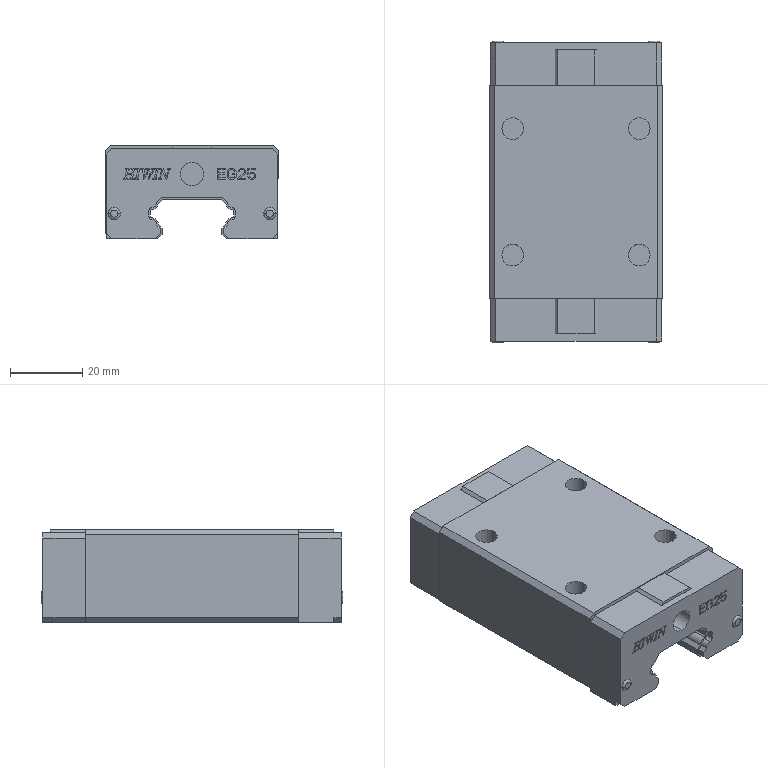Part | SolidWorks | features BaseBody 1 | 1 solid | 411 faces | box 48 x 83.6 x 26 mm | volume 72725 mm3 | plane 301 | spline 68 | cylinder 42 | commonest cylinder face diameters 4 x10 2 x8 3 x8 6 x8 1 x4 6.4 x4